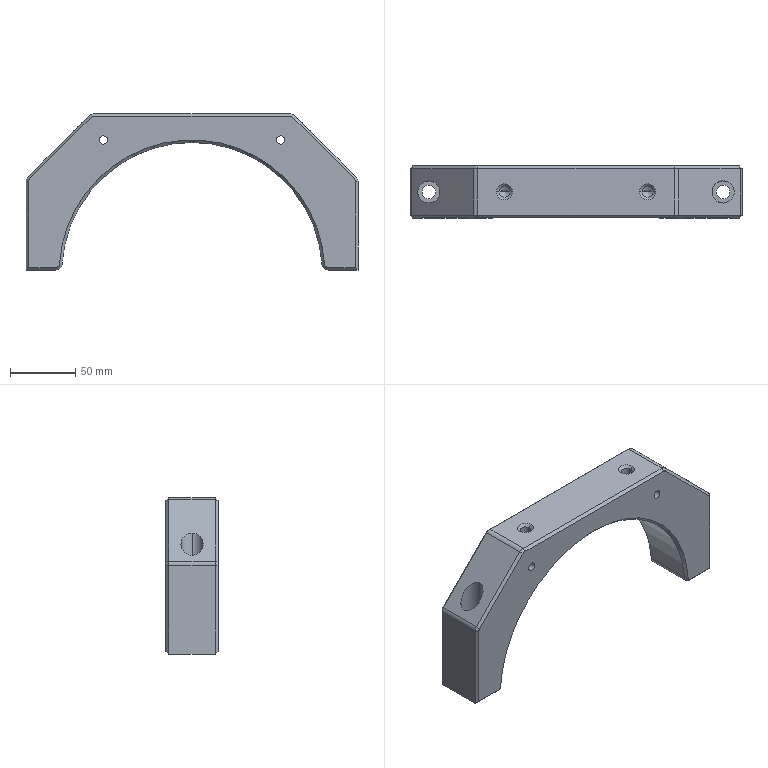Part | NX | features BREP 1 | 1 solid | 76 faces | box 255 x 40 x 120 mm | volume 475135 mm3 | plane 27 | cylinder 27 | cone 22 | commonest cylinder face diameters 10 x6 6.4 x4 8.376 x4 10.5 x4 11.2 x4 17 x4